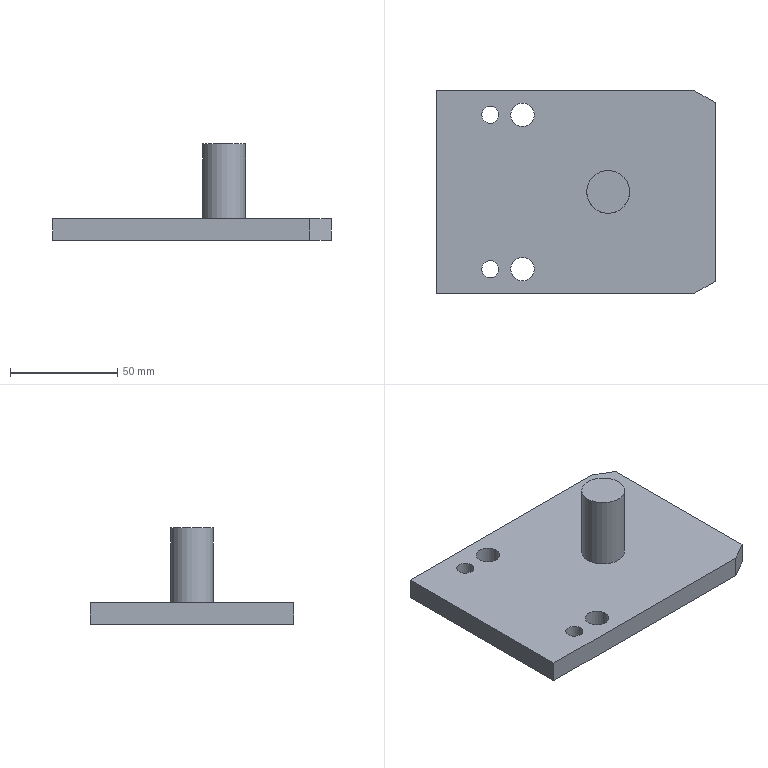Part | NX | features solid 2 | 1 solid | 14 faces | box 130 x 95 x 45 mm | volume 131012 mm3 | plane 9 | cylinder 5 | commonest cylinder face diameters 8 x2 11 x2 20 x1
STEP:
#1=CARTESIAN_POINT('',(490.903,-183.809,235.));
#2=VERTEX_POINT('',#1);
#3=CARTESIAN_POINT('',(480.903,-183.809,235.));
#4=DIRECTION('',(0.,0.,-1.));
#5=DIRECTION('',(1.,0.,0.));
#6=AXIS2_PLACEMENT_3D('',#3,#4,#5);
#7=CIRCLE('',#6,10.);
#8=EDGE_CURVE('',#2,#2,#7,.F.);
#9=ORIENTED_EDGE('',*,*,#8,.T.);
#10=EDGE_LOOP('',(#9));
#11=FACE_BOUND('',#10,.T.);
#12=CARTESIAN_POINT('',(470.903,-183.809,270.));
#13=VERTEX_POINT('',#12);
#14=CARTESIAN_POINT('',(480.903,-183.809,270.));
#15=DIRECTION('',(0.,0.,1.));
#16=DIRECTION('',(-1.,0.,0.));
#17=AXIS2_PLACEMENT_3D('',#14,#15,#16);
#18=CIRCLE('',#17,10.);
#19=EDGE_CURVE('',#13,#13,#18,.T.);
#20=ORIENTED_EDGE('',*,*,#19,.F.);
#21=EDGE_LOOP('',(#20));
#22=FACE_BOUND('',#21,.T.);
#23=CARTESIAN_POINT('',(480.903,-183.809,235.));
#24=DIRECTION('',(0.,0.,1.));
#25=DIRECTION('',(-1.,0.,0.));
#26=AXIS2_PLACEMENT_3D('',#23,#24,#25);
#27=CYLINDRICAL_SURFACE('',#26,10.);
#28=ADVANCED_FACE('',(#11,#22),#27,.T.);
#29=ORIENTED_EDGE('',*,*,#19,.T.);
#30=EDGE_LOOP('',(#29));
#31=FACE_BOUND('',#30,.T.);
#32=CARTESIAN_POINT('',(480.903,-183.809,270.));
#33=DIRECTION('',(0.,0.,1.));
#34=DIRECTION('',(-1.,0.,0.));
#35=AXIS2_PLACEMENT_3D('',#32,#33,#34);
#36=PLANE('',#35);
#37=ADVANCED_FACE('',(#31),#36,.T.);
#38=CARTESIAN_POINT('',(520.903,-136.309,225.));
#39=VERTEX_POINT('',#38);
#40=CARTESIAN_POINT('',(530.903,-142.082,225.));
#41=VERTEX_POINT('',#40);
#42=CARTESIAN_POINT('',(550.903,-153.629,225.));
#43=DIRECTION('',(-0.866,0.5,0.));
#44=VECTOR('',#43,1000.);
#45=LINE('',#42,#44);
#46=EDGE_CURVE('',#39,#41,#45,.F.);
#47=ORIENTED_EDGE('',*,*,#46,.F.);
#48=CARTESIAN_POINT('',(520.903,-136.309,235.));
#49=VERTEX_POINT('',#48);
#50=CARTESIAN_POINT('',(520.903,-136.309,235.));
#51=DIRECTION('',(0.,0.,-1.));
#52=VECTOR('',#51,1000.);
#53=LINE('',#50,#52);
#54=EDGE_CURVE('',#49,#39,#53,.T.);
#55=ORIENTED_EDGE('',*,*,#54,.F.);
#56=CARTESIAN_POINT('',(530.903,-142.082,235.));
#57=VERTEX_POINT('',#56);
#58=CARTESIAN_POINT('',(550.903,-153.629,235.));
#59=DIRECTION('',(-0.866,0.5,0.));
#60=VECTOR('',#59,1000.);
#61=LINE('',#58,#60);
#62=EDGE_CURVE('',#49,#57,#61,.F.);
#63=ORIENTED_EDGE('',*,*,#62,.T.);
#64=CARTESIAN_POINT('',(530.903,-142.082,235.));
#65=DIRECTION('',(0.,0.,-1.));
#66=VECTOR('',#65,1000.);
#67=LINE('',#64,#66);
#68=EDGE_CURVE('',#57,#41,#67,.T.);
#69=ORIENTED_EDGE('',*,*,#68,.T.);
#70=EDGE_LOOP('',(#47,#55,#63,#69));
#71=FACE_BOUND('',#70,.T.);
#72=CARTESIAN_POINT('',(550.903,-153.629,235.));
#73=DIRECTION('',(0.5,0.866,0.));
#74=DIRECTION('',(-0.866,0.5,0.));
#75=AXIS2_PLACEMENT_3D('',#72,#73,#74);
#76=PLANE('',#75);
#77=ADVANCED_FACE('',(#71),#76,.T.);
#78=CARTESIAN_POINT('',(400.903,-136.309,225.));
#79=VERTEX_POINT('',#78);
#80=CARTESIAN_POINT('',(400.903,-136.309,225.));
#81=DIRECTION('',(-1.,0.,0.));
#82=VECTOR('',#81,1000.);
#83=LINE('',#80,#82);
#84=EDGE_CURVE('',#39,#79,#83,.T.);
#85=ORIENTED_EDGE('',*,*,#84,.T.);
#86=CARTESIAN_POINT('',(400.903,-136.309,235.));
#87=VERTEX_POINT('',#86);
#88=CARTESIAN_POINT('',(400.903,-136.309,225.));
#89=DIRECTION('',(0.,0.,1.));
#90=VECTOR('',#89,1000.);
#91=LINE('',#88,#90);
#92=EDGE_CURVE('',#87,#79,#91,.F.);
#93=ORIENTED_EDGE('',*,*,#92,.F.);
#94=CARTESIAN_POINT('',(400.903,-136.309,235.));
#95=DIRECTION('',(-1.,0.,0.));
#96=VECTOR('',#95,1000.);
#97=LINE('',#94,#96);
#98=EDGE_CURVE('',#49,#87,#97,.T.);
#99=ORIENTED_EDGE('',*,*,#98,.F.);
#100=ORIENTED_EDGE('',*,*,#54,.T.);
#101=EDGE_LOOP('',(#85,#93,#99,#100));
#102=FACE_BOUND('',#101,.T.);
#103=CARTESIAN_POINT('',(400.903,-136.309,235.));
#104=DIRECTION('',(0.,-1.,0.));
#105=DIRECTION('',(1.,0.,0.));
#106=AXIS2_PLACEMENT_3D('',#103,#104,#105);
#107=PLANE('',#106);
#108=ADVANCED_FACE('',(#102),#107,.F.);
#109=CARTESIAN_POINT('',(400.903,-231.309,225.));
#110=VERTEX_POINT('',#109);
#111=CARTESIAN_POINT('',(400.903,-156.809,225.));
#112=DIRECTION('',(0.,1.,0.));
#113=VECTOR('',#112,1000.);
#114=LINE('',#111,#113);
#115=EDGE_CURVE('',#79,#110,#114,.F.);
#116=ORIENTED_EDGE('',*,*,#115,.T.);
#117=CARTESIAN_POINT('',(400.903,-231.309,235.));
#118=VERTEX_POINT('',#117);
#119=CARTESIAN_POINT('',(400.903,-231.309,225.));
#120=DIRECTION('',(0.,0.,1.));
#121=VECTOR('',#120,1000.);
#122=LINE('',#119,#121);
#123=EDGE_CURVE('',#118,#110,#122,.F.);
#124=ORIENTED_EDGE('',*,*,#123,.F.);
#125=CARTESIAN_POINT('',(400.903,-156.809,235.));
#126=DIRECTION('',(0.,1.,0.));
#127=VECTOR('',#126,1000.);
#128=LINE('',#125,#127);
#129=EDGE_CURVE('',#87,#118,#128,.F.);
#130=ORIENTED_EDGE('',*,*,#129,.F.);
#131=ORIENTED_EDGE('',*,*,#92,.T.);
#132=EDGE_LOOP('',(#116,#124,#130,#131));
#133=FACE_BOUND('',#132,.T.);
#134=CARTESIAN_POINT('',(400.903,-156.809,225.));
#135=DIRECTION('',(-1.,0.,0.));
#136=DIRECTION('',(0.,-1.,0.));
#137=AXIS2_PLACEMENT_3D('',#134,#135,#136);
#138=PLANE('',#137);
#139=ADVANCED_FACE('',(#133),#138,.T.);
#140=CARTESIAN_POINT('',(520.903,-231.309,225.));
#141=VERTEX_POINT('',#140);
#142=CARTESIAN_POINT('',(400.903,-231.309,225.));
#143=DIRECTION('',(-1.,0.,0.));
#144=VECTOR('',#143,1000.);
#145=LINE('',#142,#144);
#146=EDGE_CURVE('',#141,#110,#145,.T.);
#147=ORIENTED_EDGE('',*,*,#146,.F.);
#148=CARTESIAN_POINT('',(520.903,-231.309,235.));
#149=VERTEX_POINT('',#148);
#150=CARTESIAN_POINT('',(520.903,-231.309,235.));
#151=DIRECTION('',(0.,0.,-1.));
#152=VECTOR('',#151,1000.);
#153=LINE('',#150,#152);
#154=EDGE_CURVE('',#149,#141,#153,.T.);
#155=ORIENTED_EDGE('',*,*,#154,.F.);
#156=CARTESIAN_POINT('',(400.903,-231.309,235.));
#157=DIRECTION('',(-1.,0.,0.));
#158=VECTOR('',#157,1000.);
#159=LINE('',#156,#158);
#160=EDGE_CURVE('',#149,#118,#159,.T.);
#161=ORIENTED_EDGE('',*,*,#160,.T.);
#162=ORIENTED_EDGE('',*,*,#123,.T.);
#163=EDGE_LOOP('',(#147,#155,#161,#162));
#164=FACE_BOUND('',#163,.T.);
#165=CARTESIAN_POINT('',(400.903,-231.309,235.));
#166=DIRECTION('',(0.,-1.,0.));
#167=DIRECTION('',(1.,0.,0.));
#168=AXIS2_PLACEMENT_3D('',#165,#166,#167);
#169=PLANE('',#168);
#170=ADVANCED_FACE('',(#164),#169,.T.);
#171=CARTESIAN_POINT('',(530.903,-225.535,225.));
#172=VERTEX_POINT('',#171);
#173=CARTESIAN_POINT('',(520.903,-231.309,225.));
#174=DIRECTION('',(-0.866,-0.5,0.));
#175=VECTOR('',#174,1000.);
#176=LINE('',#173,#175);
#177=EDGE_CURVE('',#172,#141,#176,.T.);
#178=ORIENTED_EDGE('',*,*,#177,.F.);
#179=CARTESIAN_POINT('',(530.903,-225.535,235.));
#180=VERTEX_POINT('',#179);
#181=CARTESIAN_POINT('',(530.903,-225.535,235.));
#182=DIRECTION('',(0.,0.,-1.));
#183=VECTOR('',#182,1000.);
#184=LINE('',#181,#183);
#185=EDGE_CURVE('',#180,#172,#184,.T.);
#186=ORIENTED_EDGE('',*,*,#185,.F.);
#187=CARTESIAN_POINT('',(520.903,-231.309,235.));
#188=DIRECTION('',(-0.866,-0.5,0.));
#189=VECTOR('',#188,1000.);
#190=LINE('',#187,#189);
#191=EDGE_CURVE('',#180,#149,#190,.T.);
#192=ORIENTED_EDGE('',*,*,#191,.T.);
#193=ORIENTED_EDGE('',*,*,#154,.T.);
#194=EDGE_LOOP('',(#178,#186,#192,#193));
#195=FACE_BOUND('',#194,.T.);
#196=CARTESIAN_POINT('',(520.903,-231.309,235.));
#197=DIRECTION('',(0.5,-0.866,0.));
#198=DIRECTION('',(0.866,0.5,0.));
#199=AXIS2_PLACEMENT_3D('',#196,#197,#198);
#200=PLANE('',#199);
#201=ADVANCED_FACE('',(#195),#200,.T.);
#202=CARTESIAN_POINT('',(530.903,-178.809,225.));
#203=DIRECTION('',(0.,1.,0.));
#204=VECTOR('',#203,1000.);
#205=LINE('',#202,#204);
#206=EDGE_CURVE('',#172,#41,#205,.T.);
#207=ORIENTED_EDGE('',*,*,#206,.T.);
#208=ORIENTED_EDGE('',*,*,#68,.F.);
#209=CARTESIAN_POINT('',(530.903,-178.809,235.));
#210=DIRECTION('',(0.,1.,0.));
#211=VECTOR('',#210,1000.);
#212=LINE('',#209,#211);
#213=EDGE_CURVE('',#180,#57,#212,.T.);
#214=ORIENTED_EDGE('',*,*,#213,.F.);
#215=ORIENTED_EDGE('',*,*,#185,.T.);
#216=EDGE_LOOP('',(#207,#208,#214,#215));
#217=FACE_BOUND('',#216,.T.);
#218=CARTESIAN_POINT('',(530.903,-178.809,235.));
#219=DIRECTION('',(-1.,0.,0.));
#220=DIRECTION('',(0.,-1.,0.));
#221=AXIS2_PLACEMENT_3D('',#218,#219,#220);
#222=PLANE('',#221);
#223=ADVANCED_FACE('',(#217),#222,.F.);
#224=CARTESIAN_POINT('',(429.903,-147.809,235.));
#225=VERTEX_POINT('',#224);
#226=CARTESIAN_POINT('',(425.903,-147.809,235.));
#227=DIRECTION('',(0.,0.,1.));
#228=DIRECTION('',(1.,0.,0.));
#229=AXIS2_PLACEMENT_3D('',#226,#227,#228);
#230=CIRCLE('',#229,4.);
#231=EDGE_CURVE('',#225,#225,#230,.T.);
#232=ORIENTED_EDGE('',*,*,#231,.T.);
#233=EDGE_LOOP('',(#232));
#234=FACE_BOUND('',#233,.T.);
#235=CARTESIAN_POINT('',(429.903,-147.809,225.));
#236=VERTEX_POINT('',#235);
#237=CARTESIAN_POINT('',(425.903,-147.809,225.));
#238=DIRECTION('',(0.,0.,1.));
#239=DIRECTION('',(1.,0.,0.));
#240=AXIS2_PLACEMENT_3D('',#237,#238,#239);
#241=CIRCLE('',#240,4.);
#242=EDGE_CURVE('',#236,#236,#241,.T.);
#243=ORIENTED_EDGE('',*,*,#242,.F.);
#244=EDGE_LOOP('',(#243));
#245=FACE_BOUND('',#244,.T.);
#246=CARTESIAN_POINT('',(425.903,-147.809,235.));
#247=DIRECTION('',(0.,0.,-1.));
#248=DIRECTION('',(1.,0.,0.));
#249=AXIS2_PLACEMENT_3D('',#246,#247,#248);
#250=CYLINDRICAL_SURFACE('',#249,4.);
#251=ADVANCED_FACE('',(#234,#245),#250,.F.);
#252=CARTESIAN_POINT('',(429.903,-219.809,235.));
#253=VERTEX_POINT('',#252);
#254=CARTESIAN_POINT('',(425.903,-219.809,235.));
#255=DIRECTION('',(0.,0.,1.));
#256=DIRECTION('',(1.,0.,0.));
#257=AXIS2_PLACEMENT_3D('',#254,#255,#256);
#258=CIRCLE('',#257,4.);
#259=EDGE_CURVE('',#253,#253,#258,.T.);
#260=ORIENTED_EDGE('',*,*,#259,.T.);
#261=EDGE_LOOP('',(#260));
#262=FACE_BOUND('',#261,.T.);
#263=CARTESIAN_POINT('',(429.903,-219.809,225.));
#264=VERTEX_POINT('',#263);
#265=CARTESIAN_POINT('',(425.903,-219.809,225.));
#266=DIRECTION('',(0.,0.,1.));
#267=DIRECTION('',(1.,0.,0.));
#268=AXIS2_PLACEMENT_3D('',#265,#266,#267);
#269=CIRCLE('',#268,4.);
#270=EDGE_CURVE('',#264,#264,#269,.T.);
#271=ORIENTED_EDGE('',*,*,#270,.F.);
#272=EDGE_LOOP('',(#271));
#273=FACE_BOUND('',#272,.T.);
#274=CARTESIAN_POINT('',(425.903,-219.809,235.));
#275=DIRECTION('',(0.,0.,-1.));
#276=DIRECTION('',(1.,0.,0.));
#277=AXIS2_PLACEMENT_3D('',#274,#275,#276);
#278=CYLINDRICAL_SURFACE('',#277,4.);
#279=ADVANCED_FACE('',(#262,#273),#278,.F.);
#280=CARTESIAN_POINT('',(446.403,-219.809,235.));
#281=VERTEX_POINT('',#280);
#282=CARTESIAN_POINT('',(440.903,-219.809,235.));
#283=DIRECTION('',(0.,0.,-1.));
#284=DIRECTION('',(1.,0.,0.));
#285=AXIS2_PLACEMENT_3D('',#282,#283,#284);
#286=CIRCLE('',#285,5.5);
#287=EDGE_CURVE('',#281,#281,#286,.F.);
#288=ORIENTED_EDGE('',*,*,#287,.T.);
#289=EDGE_LOOP('',(#288));
#290=FACE_BOUND('',#289,.T.);
#291=CARTESIAN_POINT('',(446.403,-219.809,225.));
#292=VERTEX_POINT('',#291);
#293=CARTESIAN_POINT('',(440.903,-219.809,225.));
#294=DIRECTION('',(0.,0.,-1.));
#295=DIRECTION('',(1.,0.,0.));
#296=AXIS2_PLACEMENT_3D('',#293,#294,#295);
#297=CIRCLE('',#296,5.5);
#298=EDGE_CURVE('',#292,#292,#297,.F.);
#299=ORIENTED_EDGE('',*,*,#298,.F.);
#300=EDGE_LOOP('',(#299));
#301=FACE_BOUND('',#300,.T.);
#302=CARTESIAN_POINT('',(440.903,-219.809,235.));
#303=DIRECTION('',(0.,0.,-1.));
#304=DIRECTION('',(1.,0.,0.));
#305=AXIS2_PLACEMENT_3D('',#302,#303,#304);
#306=CYLINDRICAL_SURFACE('',#305,5.5);
#307=ADVANCED_FACE('',(#290,#301),#306,.F.);
#308=CARTESIAN_POINT('',(446.403,-147.809,235.));
#309=VERTEX_POINT('',#308);
#310=CARTESIAN_POINT('',(440.903,-147.809,235.));
#311=DIRECTION('',(0.,0.,-1.));
#312=DIRECTION('',(1.,0.,0.));
#313=AXIS2_PLACEMENT_3D('',#310,#311,#312);
#314=CIRCLE('',#313,5.5);
#315=EDGE_CURVE('',#309,#309,#314,.F.);
#316=ORIENTED_EDGE('',*,*,#315,.T.);
#317=EDGE_LOOP('',(#316));
#318=FACE_BOUND('',#317,.T.);
#319=CARTESIAN_POINT('',(446.403,-147.809,225.));
#320=VERTEX_POINT('',#319);
#321=CARTESIAN_POINT('',(440.903,-147.809,225.));
#322=DIRECTION('',(0.,0.,-1.));
#323=DIRECTION('',(1.,0.,0.));
#324=AXIS2_PLACEMENT_3D('',#321,#322,#323);
#325=CIRCLE('',#324,5.5);
#326=EDGE_CURVE('',#320,#320,#325,.F.);
#327=ORIENTED_EDGE('',*,*,#326,.F.);
#328=EDGE_LOOP('',(#327));
#329=FACE_BOUND('',#328,.T.);
#330=CARTESIAN_POINT('',(440.903,-147.809,235.));
#331=DIRECTION('',(0.,0.,-1.));
#332=DIRECTION('',(1.,0.,0.));
#333=AXIS2_PLACEMENT_3D('',#330,#331,#332);
#334=CYLINDRICAL_SURFACE('',#333,5.5);
#335=ADVANCED_FACE('',(#318,#329),#334,.F.);
#336=ORIENTED_EDGE('',*,*,#8,.F.);
#337=EDGE_LOOP('',(#336));
#338=FACE_BOUND('',#337,.T.);
#339=ORIENTED_EDGE('',*,*,#191,.F.);
#340=ORIENTED_EDGE('',*,*,#213,.T.);
#341=ORIENTED_EDGE('',*,*,#62,.F.);
#342=ORIENTED_EDGE('',*,*,#98,.T.);
#343=ORIENTED_EDGE('',*,*,#129,.T.);
#344=ORIENTED_EDGE('',*,*,#160,.F.);
#345=EDGE_LOOP('',(#339,#340,#341,#342,#343,#344));
#346=FACE_BOUND('',#345,.T.);
#347=ORIENTED_EDGE('',*,*,#287,.F.);
#348=EDGE_LOOP('',(#347));
#349=FACE_BOUND('',#348,.T.);
#350=ORIENTED_EDGE('',*,*,#259,.F.);
#351=EDGE_LOOP('',(#350));
#352=FACE_BOUND('',#351,.T.);
#353=ORIENTED_EDGE('',*,*,#231,.F.);
#354=EDGE_LOOP('',(#353));
#355=FACE_BOUND('',#354,.T.);
#356=ORIENTED_EDGE('',*,*,#315,.F.);
#357=EDGE_LOOP('',(#356));
#358=FACE_BOUND('',#357,.T.);
#359=CARTESIAN_POINT('',(400.903,-156.809,235.));
#360=DIRECTION('',(0.,0.,-1.));
#361=DIRECTION('',(1.,0.,0.));
#362=AXIS2_PLACEMENT_3D('',#359,#360,#361);
#363=PLANE('',#362);
#364=ADVANCED_FACE('',(#338,#346,#349,#352,#355,#358),#363,.F.);
#365=ORIENTED_EDGE('',*,*,#46,.T.);
#366=ORIENTED_EDGE('',*,*,#206,.F.);
#367=ORIENTED_EDGE('',*,*,#177,.T.);
#368=ORIENTED_EDGE('',*,*,#146,.T.);
#369=ORIENTED_EDGE('',*,*,#115,.F.);
#370=ORIENTED_EDGE('',*,*,#84,.F.);
#371=EDGE_LOOP('',(#365,#366,#367,#368,#369,#370));
#372=FACE_BOUND('',#371,.T.);
#373=ORIENTED_EDGE('',*,*,#298,.T.);
#374=EDGE_LOOP('',(#373));
#375=FACE_BOUND('',#374,.T.);
#376=ORIENTED_EDGE('',*,*,#270,.T.);
#377=EDGE_LOOP('',(#376));
#378=FACE_BOUND('',#377,.T.);
#379=ORIENTED_EDGE('',*,*,#242,.T.);
#380=EDGE_LOOP('',(#379));
#381=FACE_BOUND('',#380,.T.);
#382=ORIENTED_EDGE('',*,*,#326,.T.);
#383=EDGE_LOOP('',(#382));
#384=FACE_BOUND('',#383,.T.);
#385=CARTESIAN_POINT('',(400.903,-156.809,225.));
#386=DIRECTION('',(0.,0.,-1.));
#387=DIRECTION('',(1.,0.,0.));
#388=AXIS2_PLACEMENT_3D('',#385,#386,#387);
#389=PLANE('',#388);
#390=ADVANCED_FACE('',(#372,#375,#378,#381,#384),#389,.T.);
#391=CLOSED_SHELL('',(#28,#37,#77,#108,#139,#170,#201,#223,#251,#279,#307,#335,#364,#390));
#392=MANIFOLD_SOLID_BREP('',#391);
#393=(LENGTH_UNIT()NAMED_UNIT(*)SI_UNIT(.MILLI.,.METRE.));
#394=UNCERTAINTY_MEASURE_WITH_UNIT(LENGTH_MEASURE(0.00001),#393,'','');
#395=(NAMED_UNIT(*)PLANE_ANGLE_UNIT()SI_UNIT($,.RADIAN.));
#396=(NAMED_UNIT(*)SI_UNIT($,.STERADIAN.)SOLID_ANGLE_UNIT());
#397=(GEOMETRIC_REPRESENTATION_CONTEXT(3)GLOBAL_UNCERTAINTY_ASSIGNED_CONTEXT((#394))GLOBAL_UNIT_ASSIGNED_CONTEXT((#393,#395,#396))REPRESENTATION_CONTEXT('',''));
#398=ADVANCED_BREP_SHAPE_REPRESENTATION('',(#392),#397);